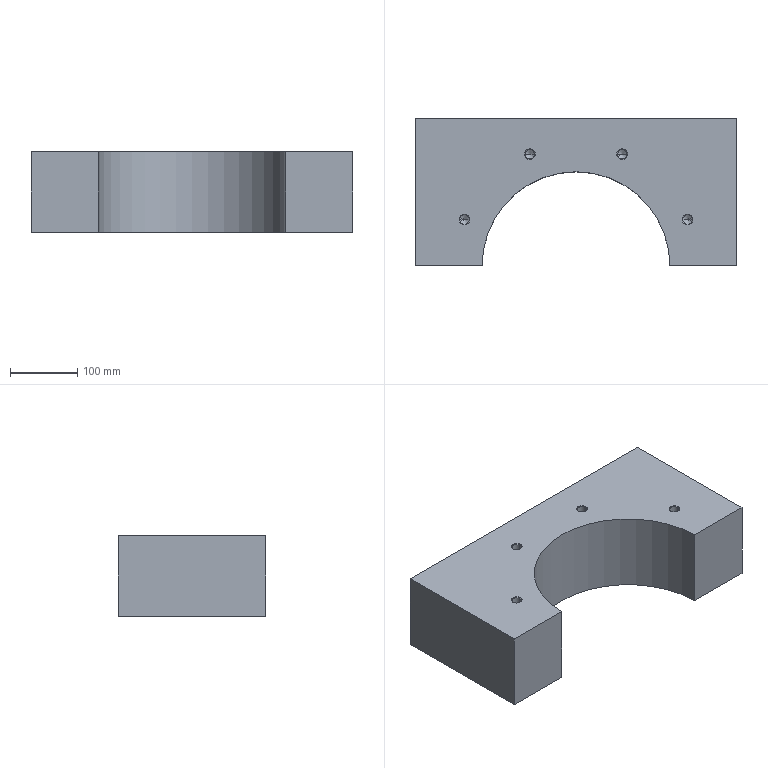Part | SolidWorks | features Extrusion 1, HoleWzd 1, RefAxis 1 | 1 solid | 32 faces | box 480 x 220 x 120 mm | volume 8956950 mm3 | cone 16 | cylinder 9 | plane 7 | commonest cylinder face diameters 14 x8 280 x1
STEP:
#1=CARTESIAN_POINT('',(-173.298,68.883,118.975));
#2=VERTEX_POINT('',#1);
#3=CARTESIAN_POINT('',(-159.298,68.883,118.975));
#4=VERTEX_POINT('',#3);
#5=CARTESIAN_POINT('',(-166.298,68.883,118.975));
#6=DIRECTION('',(0.,0.,1.));
#7=DIRECTION('',(1.,0.,0.));
#8=AXIS2_PLACEMENT_3D('',#5,#6,#7);
#9=CIRCLE('',#8,7.);
#10=EDGE_CURVE('',#2,#4,#9,.T.);
#11=ORIENTED_EDGE('',*,*,#10,.F.);
#12=CARTESIAN_POINT('',(-174.323,68.883,120.));
#13=VERTEX_POINT('',#12);
#14=CARTESIAN_POINT('',(-174.323,68.883,120.));
#15=DIRECTION('',(-0.7071,0.,0.7071));
#16=VECTOR('',#15,1000.);
#17=LINE('',#14,#16);
#18=EDGE_CURVE('',#2,#13,#17,.T.);
#19=ORIENTED_EDGE('',*,*,#18,.T.);
#20=CARTESIAN_POINT('',(-158.273,68.883,120.));
#21=VERTEX_POINT('',#20);
#22=CARTESIAN_POINT('',(-166.298,68.883,120.));
#23=DIRECTION('',(0.,0.,1.));
#24=DIRECTION('',(1.,0.,0.));
#25=AXIS2_PLACEMENT_3D('',#22,#23,#24);
#26=CIRCLE('',#25,8.025);
#27=EDGE_CURVE('',#13,#21,#26,.T.);
#28=ORIENTED_EDGE('',*,*,#27,.T.);
#29=CARTESIAN_POINT('',(-158.273,68.883,120.));
#30=DIRECTION('',(0.7071,0.,0.7071));
#31=VECTOR('',#30,1000.);
#32=LINE('',#29,#31);
#33=EDGE_CURVE('',#4,#21,#32,.T.);
#34=ORIENTED_EDGE('',*,*,#33,.F.);
#35=EDGE_LOOP('',(#11,#19,#28,#34));
#36=FACE_OUTER_BOUND('',#35,.T.);
#37=CARTESIAN_POINT('',(-166.298,68.883,120.));
#38=DIRECTION('',(0.,0.,1.));
#39=DIRECTION('',(1.,0.,0.));
#40=AXIS2_PLACEMENT_3D('',#37,#38,#39);
#41=CONICAL_SURFACE('',#40,8.025,0.7854);
#42=ADVANCED_FACE('',(#36),#41,.F.);
#43=CARTESIAN_POINT('',(-173.298,68.883,88.206));
#44=VERTEX_POINT('',#43);
#45=CARTESIAN_POINT('',(-159.298,68.883,88.206));
#46=VERTEX_POINT('',#45);
#47=CARTESIAN_POINT('',(-166.298,68.883,88.206));
#48=DIRECTION('',(0.,0.,1.));
#49=DIRECTION('',(1.,0.,0.));
#50=AXIS2_PLACEMENT_3D('',#47,#48,#49);
#51=CIRCLE('',#50,7.);
#52=EDGE_CURVE('',#44,#46,#51,.T.);
#53=ORIENTED_EDGE('',*,*,#52,.F.);
#54=CARTESIAN_POINT('',(-173.298,68.883,120.));
#55=DIRECTION('',(0.,0.,1.));
#56=VECTOR('',#55,1000.);
#57=LINE('',#54,#56);
#58=EDGE_CURVE('',#44,#2,#57,.T.);
#59=ORIENTED_EDGE('',*,*,#58,.T.);
#60=ORIENTED_EDGE('',*,*,#10,.T.);
#61=CARTESIAN_POINT('',(-159.298,68.883,120.));
#62=DIRECTION('',(0.,0.,1.));
#63=VECTOR('',#62,1000.);
#64=LINE('',#61,#63);
#65=EDGE_CURVE('',#46,#4,#64,.T.);
#66=ORIENTED_EDGE('',*,*,#65,.F.);
#67=EDGE_LOOP('',(#53,#59,#60,#66));
#68=FACE_OUTER_BOUND('',#67,.T.);
#69=CARTESIAN_POINT('',(-166.298,68.883,120.));
#70=DIRECTION('',(0.,0.,1.));
#71=DIRECTION('',(1.,0.,0.));
#72=AXIS2_PLACEMENT_3D('',#69,#70,#71);
#73=CYLINDRICAL_SURFACE('',#72,7.);
#74=ADVANCED_FACE('',(#68),#73,.F.);
#75=CARTESIAN_POINT('',(-166.298,68.883,84.));
#76=VERTEX_POINT('',#75);
#77=CARTESIAN_POINT('',(-159.298,68.883,88.206));
#78=DIRECTION('',(0.8572,0.,0.515));
#79=VECTOR('',#78,1000.);
#80=LINE('',#77,#79);
#81=EDGE_CURVE('',#76,#46,#80,.T.);
#82=ORIENTED_EDGE('',*,*,#81,.F.);
#83=CARTESIAN_POINT('',(-173.298,68.883,88.206));
#84=DIRECTION('',(-0.8572,0.,0.515));
#85=VECTOR('',#84,1000.);
#86=LINE('',#83,#85);
#87=EDGE_CURVE('',#76,#44,#86,.T.);
#88=ORIENTED_EDGE('',*,*,#87,.T.);
#89=ORIENTED_EDGE('',*,*,#52,.T.);
#90=EDGE_LOOP('',(#82,#88,#89));
#91=FACE_OUTER_BOUND('',#90,.T.);
#92=CARTESIAN_POINT('',(-166.298,68.883,88.206));
#93=DIRECTION('',(0.,0.,1.));
#94=DIRECTION('',(1.,0.,0.));
#95=AXIS2_PLACEMENT_3D('',#92,#93,#94);
#96=CONICAL_SURFACE('',#95,7.,1.03);
#97=ADVANCED_FACE('',(#91),#96,.F.);
#98=CARTESIAN_POINT('',(-75.883,166.298,118.975));
#99=VERTEX_POINT('',#98);
#100=CARTESIAN_POINT('',(-61.883,166.298,118.975));
#101=VERTEX_POINT('',#100);
#102=CARTESIAN_POINT('',(-68.883,166.298,118.975));
#103=DIRECTION('',(0.,0.,1.));
#104=DIRECTION('',(1.,0.,0.));
#105=AXIS2_PLACEMENT_3D('',#102,#103,#104);
#106=CIRCLE('',#105,7.);
#107=EDGE_CURVE('',#99,#101,#106,.T.);
#108=ORIENTED_EDGE('',*,*,#107,.F.);
#109=CARTESIAN_POINT('',(-76.908,166.298,120.));
#110=VERTEX_POINT('',#109);
#111=CARTESIAN_POINT('',(-76.908,166.298,120.));
#112=DIRECTION('',(-0.7071,0.,0.7071));
#113=VECTOR('',#112,1000.);
#114=LINE('',#111,#113);
#115=EDGE_CURVE('',#99,#110,#114,.T.);
#116=ORIENTED_EDGE('',*,*,#115,.T.);
#117=CARTESIAN_POINT('',(-60.858,166.298,120.));
#118=VERTEX_POINT('',#117);
#119=CARTESIAN_POINT('',(-68.883,166.298,120.));
#120=DIRECTION('',(0.,0.,1.));
#121=DIRECTION('',(1.,0.,0.));
#122=AXIS2_PLACEMENT_3D('',#119,#120,#121);
#123=CIRCLE('',#122,8.025);
#124=EDGE_CURVE('',#110,#118,#123,.T.);
#125=ORIENTED_EDGE('',*,*,#124,.T.);
#126=CARTESIAN_POINT('',(-60.858,166.298,120.));
#127=DIRECTION('',(0.7071,0.,0.7071));
#128=VECTOR('',#127,1000.);
#129=LINE('',#126,#128);
#130=EDGE_CURVE('',#101,#118,#129,.T.);
#131=ORIENTED_EDGE('',*,*,#130,.F.);
#132=EDGE_LOOP('',(#108,#116,#125,#131));
#133=FACE_OUTER_BOUND('',#132,.T.);
#134=CARTESIAN_POINT('',(-68.883,166.298,120.));
#135=DIRECTION('',(0.,0.,1.));
#136=DIRECTION('',(1.,0.,0.));
#137=AXIS2_PLACEMENT_3D('',#134,#135,#136);
#138=CONICAL_SURFACE('',#137,8.025,0.7854);
#139=ADVANCED_FACE('',(#133),#138,.F.);
#140=CARTESIAN_POINT('',(-75.883,166.298,88.206));
#141=VERTEX_POINT('',#140);
#142=CARTESIAN_POINT('',(-61.883,166.298,88.206));
#143=VERTEX_POINT('',#142);
#144=CARTESIAN_POINT('',(-68.883,166.298,88.206));
#145=DIRECTION('',(0.,0.,1.));
#146=DIRECTION('',(1.,0.,0.));
#147=AXIS2_PLACEMENT_3D('',#144,#145,#146);
#148=CIRCLE('',#147,7.);
#149=EDGE_CURVE('',#141,#143,#148,.T.);
#150=ORIENTED_EDGE('',*,*,#149,.F.);
#151=CARTESIAN_POINT('',(-75.883,166.298,120.));
#152=DIRECTION('',(0.,0.,1.));
#153=VECTOR('',#152,1000.);
#154=LINE('',#151,#153);
#155=EDGE_CURVE('',#141,#99,#154,.T.);
#156=ORIENTED_EDGE('',*,*,#155,.T.);
#157=ORIENTED_EDGE('',*,*,#107,.T.);
#158=CARTESIAN_POINT('',(-61.883,166.298,120.));
#159=DIRECTION('',(0.,0.,1.));
#160=VECTOR('',#159,1000.);
#161=LINE('',#158,#160);
#162=EDGE_CURVE('',#143,#101,#161,.T.);
#163=ORIENTED_EDGE('',*,*,#162,.F.);
#164=EDGE_LOOP('',(#150,#156,#157,#163));
#165=FACE_OUTER_BOUND('',#164,.T.);
#166=CARTESIAN_POINT('',(-68.883,166.298,120.));
#167=DIRECTION('',(0.,0.,1.));
#168=DIRECTION('',(1.,0.,0.));
#169=AXIS2_PLACEMENT_3D('',#166,#167,#168);
#170=CYLINDRICAL_SURFACE('',#169,7.);
#171=ADVANCED_FACE('',(#165),#170,.F.);
#172=CARTESIAN_POINT('',(-68.883,166.298,84.));
#173=VERTEX_POINT('',#172);
#174=CARTESIAN_POINT('',(-61.883,166.298,88.206));
#175=DIRECTION('',(0.8572,0.,0.515));
#176=VECTOR('',#175,1000.);
#177=LINE('',#174,#176);
#178=EDGE_CURVE('',#173,#143,#177,.T.);
#179=ORIENTED_EDGE('',*,*,#178,.F.);
#180=CARTESIAN_POINT('',(-75.883,166.298,88.206));
#181=DIRECTION('',(-0.8572,0.,0.515));
#182=VECTOR('',#181,1000.);
#183=LINE('',#180,#182);
#184=EDGE_CURVE('',#173,#141,#183,.T.);
#185=ORIENTED_EDGE('',*,*,#184,.T.);
#186=ORIENTED_EDGE('',*,*,#149,.T.);
#187=EDGE_LOOP('',(#179,#185,#186));
#188=FACE_OUTER_BOUND('',#187,.T.);
#189=CARTESIAN_POINT('',(-68.883,166.298,88.206));
#190=DIRECTION('',(0.,0.,1.));
#191=DIRECTION('',(1.,0.,0.));
#192=AXIS2_PLACEMENT_3D('',#189,#190,#191);
#193=CONICAL_SURFACE('',#192,7.,1.03);
#194=ADVANCED_FACE('',(#188),#193,.F.);
#195=CARTESIAN_POINT('',(61.883,166.298,118.975));
#196=VERTEX_POINT('',#195);
#197=CARTESIAN_POINT('',(75.883,166.298,118.975));
#198=VERTEX_POINT('',#197);
#199=CARTESIAN_POINT('',(68.883,166.298,118.975));
#200=DIRECTION('',(0.,0.,1.));
#201=DIRECTION('',(1.,0.,0.));
#202=AXIS2_PLACEMENT_3D('',#199,#200,#201);
#203=CIRCLE('',#202,7.);
#204=EDGE_CURVE('',#196,#198,#203,.T.);
#205=ORIENTED_EDGE('',*,*,#204,.F.);
#206=CARTESIAN_POINT('',(60.858,166.298,120.));
#207=VERTEX_POINT('',#206);
#208=CARTESIAN_POINT('',(60.858,166.298,120.));
#209=DIRECTION('',(-0.7071,0.,0.7071));
#210=VECTOR('',#209,1000.);
#211=LINE('',#208,#210);
#212=EDGE_CURVE('',#196,#207,#211,.T.);
#213=ORIENTED_EDGE('',*,*,#212,.T.);
#214=CARTESIAN_POINT('',(76.908,166.298,120.));
#215=VERTEX_POINT('',#214);
#216=CARTESIAN_POINT('',(68.883,166.298,120.));
#217=DIRECTION('',(0.,0.,1.));
#218=DIRECTION('',(1.,0.,0.));
#219=AXIS2_PLACEMENT_3D('',#216,#217,#218);
#220=CIRCLE('',#219,8.025);
#221=EDGE_CURVE('',#207,#215,#220,.T.);
#222=ORIENTED_EDGE('',*,*,#221,.T.);
#223=CARTESIAN_POINT('',(76.908,166.298,120.));
#224=DIRECTION('',(0.7071,0.,0.7071));
#225=VECTOR('',#224,1000.);
#226=LINE('',#223,#225);
#227=EDGE_CURVE('',#198,#215,#226,.T.);
#228=ORIENTED_EDGE('',*,*,#227,.F.);
#229=EDGE_LOOP('',(#205,#213,#222,#228));
#230=FACE_OUTER_BOUND('',#229,.T.);
#231=CARTESIAN_POINT('',(68.883,166.298,120.));
#232=DIRECTION('',(0.,0.,1.));
#233=DIRECTION('',(1.,0.,0.));
#234=AXIS2_PLACEMENT_3D('',#231,#232,#233);
#235=CONICAL_SURFACE('',#234,8.025,0.7854);
#236=ADVANCED_FACE('',(#230),#235,.F.);
#237=CARTESIAN_POINT('',(61.883,166.298,88.206));
#238=VERTEX_POINT('',#237);
#239=CARTESIAN_POINT('',(75.883,166.298,88.206));
#240=VERTEX_POINT('',#239);
#241=CARTESIAN_POINT('',(68.883,166.298,88.206));
#242=DIRECTION('',(0.,0.,1.));
#243=DIRECTION('',(1.,0.,0.));
#244=AXIS2_PLACEMENT_3D('',#241,#242,#243);
#245=CIRCLE('',#244,7.);
#246=EDGE_CURVE('',#238,#240,#245,.T.);
#247=ORIENTED_EDGE('',*,*,#246,.F.);
#248=CARTESIAN_POINT('',(61.883,166.298,120.));
#249=DIRECTION('',(0.,0.,1.));
#250=VECTOR('',#249,1000.);
#251=LINE('',#248,#250);
#252=EDGE_CURVE('',#238,#196,#251,.T.);
#253=ORIENTED_EDGE('',*,*,#252,.T.);
#254=ORIENTED_EDGE('',*,*,#204,.T.);
#255=CARTESIAN_POINT('',(75.883,166.298,120.));
#256=DIRECTION('',(0.,0.,1.));
#257=VECTOR('',#256,1000.);
#258=LINE('',#255,#257);
#259=EDGE_CURVE('',#240,#198,#258,.T.);
#260=ORIENTED_EDGE('',*,*,#259,.F.);
#261=EDGE_LOOP('',(#247,#253,#254,#260));
#262=FACE_OUTER_BOUND('',#261,.T.);
#263=CARTESIAN_POINT('',(68.883,166.298,120.));
#264=DIRECTION('',(0.,0.,1.));
#265=DIRECTION('',(1.,0.,0.));
#266=AXIS2_PLACEMENT_3D('',#263,#264,#265);
#267=CYLINDRICAL_SURFACE('',#266,7.);
#268=ADVANCED_FACE('',(#262),#267,.F.);
#269=CARTESIAN_POINT('',(68.883,166.298,84.));
#270=VERTEX_POINT('',#269);
#271=CARTESIAN_POINT('',(75.883,166.298,88.206));
#272=DIRECTION('',(0.8572,0.,0.515));
#273=VECTOR('',#272,1000.);
#274=LINE('',#271,#273);
#275=EDGE_CURVE('',#270,#240,#274,.T.);
#276=ORIENTED_EDGE('',*,*,#275,.F.);
#277=CARTESIAN_POINT('',(61.883,166.298,88.206));
#278=DIRECTION('',(-0.8572,0.,0.515));
#279=VECTOR('',#278,1000.);
#280=LINE('',#277,#279);
#281=EDGE_CURVE('',#270,#238,#280,.T.);
#282=ORIENTED_EDGE('',*,*,#281,.T.);
#283=ORIENTED_EDGE('',*,*,#246,.T.);
#284=EDGE_LOOP('',(#276,#282,#283));
#285=FACE_OUTER_BOUND('',#284,.T.);
#286=CARTESIAN_POINT('',(68.883,166.298,88.206));
#287=DIRECTION('',(0.,0.,1.));
#288=DIRECTION('',(1.,0.,0.));
#289=AXIS2_PLACEMENT_3D('',#286,#287,#288);
#290=CONICAL_SURFACE('',#289,7.,1.03);
#291=ADVANCED_FACE('',(#285),#290,.F.);
#292=CARTESIAN_POINT('',(159.298,68.883,118.975));
#293=VERTEX_POINT('',#292);
#294=CARTESIAN_POINT('',(173.298,68.883,118.975));
#295=VERTEX_POINT('',#294);
#296=CARTESIAN_POINT('',(166.298,68.883,118.975));
#297=DIRECTION('',(0.,0.,1.));
#298=DIRECTION('',(1.,0.,0.));
#299=AXIS2_PLACEMENT_3D('',#296,#297,#298);
#300=CIRCLE('',#299,7.);
#301=EDGE_CURVE('',#293,#295,#300,.T.);
#302=ORIENTED_EDGE('',*,*,#301,.F.);
#303=CARTESIAN_POINT('',(158.273,68.883,120.));
#304=VERTEX_POINT('',#303);
#305=CARTESIAN_POINT('',(158.273,68.883,120.));
#306=DIRECTION('',(-0.7071,0.,0.7071));
#307=VECTOR('',#306,1000.);
#308=LINE('',#305,#307);
#309=EDGE_CURVE('',#293,#304,#308,.T.);
#310=ORIENTED_EDGE('',*,*,#309,.T.);
#311=CARTESIAN_POINT('',(174.323,68.883,120.));
#312=VERTEX_POINT('',#311);
#313=CARTESIAN_POINT('',(166.298,68.883,120.));
#314=DIRECTION('',(0.,0.,1.));
#315=DIRECTION('',(1.,0.,0.));
#316=AXIS2_PLACEMENT_3D('',#313,#314,#315);
#317=CIRCLE('',#316,8.025);
#318=EDGE_CURVE('',#304,#312,#317,.T.);
#319=ORIENTED_EDGE('',*,*,#318,.T.);
#320=CARTESIAN_POINT('',(174.323,68.883,120.));
#321=DIRECTION('',(0.7071,0.,0.7071));
#322=VECTOR('',#321,1000.);
#323=LINE('',#320,#322);
#324=EDGE_CURVE('',#295,#312,#323,.T.);
#325=ORIENTED_EDGE('',*,*,#324,.F.);
#326=EDGE_LOOP('',(#302,#310,#319,#325));
#327=FACE_OUTER_BOUND('',#326,.T.);
#328=CARTESIAN_POINT('',(166.298,68.883,120.));
#329=DIRECTION('',(0.,0.,1.));
#330=DIRECTION('',(1.,0.,0.));
#331=AXIS2_PLACEMENT_3D('',#328,#329,#330);
#332=CONICAL_SURFACE('',#331,8.025,0.7854);
#333=ADVANCED_FACE('',(#327),#332,.F.);
#334=CARTESIAN_POINT('',(159.298,68.883,88.206));
#335=VERTEX_POINT('',#334);
#336=CARTESIAN_POINT('',(173.298,68.883,88.206));
#337=VERTEX_POINT('',#336);
#338=CARTESIAN_POINT('',(166.298,68.883,88.206));
#339=DIRECTION('',(0.,0.,1.));
#340=DIRECTION('',(1.,0.,0.));
#341=AXIS2_PLACEMENT_3D('',#338,#339,#340);
#342=CIRCLE('',#341,7.);
#343=EDGE_CURVE('',#335,#337,#342,.T.);
#344=ORIENTED_EDGE('',*,*,#343,.F.);
#345=CARTESIAN_POINT('',(159.298,68.883,120.));
#346=DIRECTION('',(0.,0.,1.));
#347=VECTOR('',#346,1000.);
#348=LINE('',#345,#347);
#349=EDGE_CURVE('',#335,#293,#348,.T.);
#350=ORIENTED_EDGE('',*,*,#349,.T.);
#351=ORIENTED_EDGE('',*,*,#301,.T.);
#352=CARTESIAN_POINT('',(173.298,68.883,120.));
#353=DIRECTION('',(0.,0.,1.));
#354=VECTOR('',#353,1000.);
#355=LINE('',#352,#354);
#356=EDGE_CURVE('',#337,#295,#355,.T.);
#357=ORIENTED_EDGE('',*,*,#356,.F.);
#358=EDGE_LOOP('',(#344,#350,#351,#357));
#359=FACE_OUTER_BOUND('',#358,.T.);
#360=CARTESIAN_POINT('',(166.298,68.883,120.));
#361=DIRECTION('',(0.,0.,1.));
#362=DIRECTION('',(1.,0.,0.));
#363=AXIS2_PLACEMENT_3D('',#360,#361,#362);
#364=CYLINDRICAL_SURFACE('',#363,7.);
#365=ADVANCED_FACE('',(#359),#364,.F.);
#366=CARTESIAN_POINT('',(166.298,68.883,84.));
#367=VERTEX_POINT('',#366);
#368=CARTESIAN_POINT('',(173.298,68.883,88.206));
#369=DIRECTION('',(0.8572,0.,0.515));
#370=VECTOR('',#369,1000.);
#371=LINE('',#368,#370);
#372=EDGE_CURVE('',#367,#337,#371,.T.);
#373=ORIENTED_EDGE('',*,*,#372,.F.);
#374=CARTESIAN_POINT('',(159.298,68.883,88.206));
#375=DIRECTION('',(-0.8572,0.,0.515));
#376=VECTOR('',#375,1000.);
#377=LINE('',#374,#376);
#378=EDGE_CURVE('',#367,#335,#377,.T.);
#379=ORIENTED_EDGE('',*,*,#378,.T.);
#380=ORIENTED_EDGE('',*,*,#343,.T.);
#381=EDGE_LOOP('',(#373,#379,#380));
#382=FACE_OUTER_BOUND('',#381,.T.);
#383=CARTESIAN_POINT('',(166.298,68.883,88.206));
#384=DIRECTION('',(0.,0.,1.));
#385=DIRECTION('',(1.,0.,0.));
#386=AXIS2_PLACEMENT_3D('',#383,#384,#385);
#387=CONICAL_SURFACE('',#386,7.,1.03);
#388=ADVANCED_FACE('',(#382),#387,.F.);
#389=CARTESIAN_POINT('',(140.,0.,0.));
#390=VERTEX_POINT('',#389);
#391=CARTESIAN_POINT('',(240.,0.,0.));
#392=VERTEX_POINT('',#391);
#393=CARTESIAN_POINT('',(140.,0.,0.));
#394=DIRECTION('',(1.,0.,0.));
#395=VECTOR('',#394,1000.);
#396=LINE('',#393,#395);
#397=EDGE_CURVE('',#390,#392,#396,.T.);
#398=ORIENTED_EDGE('',*,*,#397,.T.);
#399=CARTESIAN_POINT('',(240.,0.,120.));
#400=VERTEX_POINT('',#399);
#401=CARTESIAN_POINT('',(240.,0.,120.));
#402=DIRECTION('',(0.,0.,-1.));
#403=VECTOR('',#402,1000.);
#404=LINE('',#401,#403);
#405=EDGE_CURVE('',#400,#392,#404,.T.);
#406=ORIENTED_EDGE('',*,*,#405,.F.);
#407=CARTESIAN_POINT('',(140.,0.,120.));
#408=VERTEX_POINT('',#407);
#409=CARTESIAN_POINT('',(140.,0.,120.));
#410=DIRECTION('',(1.,0.,0.));
#411=VECTOR('',#410,1000.);
#412=LINE('',#409,#411);
#413=EDGE_CURVE('',#408,#400,#412,.T.);
#414=ORIENTED_EDGE('',*,*,#413,.F.);
#415=CARTESIAN_POINT('',(140.,0.,120.));
#416=DIRECTION('',(0.,0.,-1.));
#417=VECTOR('',#416,1000.);
#418=LINE('',#415,#417);
#419=EDGE_CURVE('',#408,#390,#418,.T.);
#420=ORIENTED_EDGE('',*,*,#419,.T.);
#421=EDGE_LOOP('',(#398,#406,#414,#420));
#422=FACE_OUTER_BOUND('',#421,.T.);
#423=CARTESIAN_POINT('',(140.,0.,120.));
#424=DIRECTION('',(0.,1.,0.));
#425=DIRECTION('',(0.,0.,1.));
#426=AXIS2_PLACEMENT_3D('',#423,#424,#425);
#427=PLANE('',#426);
#428=ADVANCED_FACE('',(#422),#427,.F.);
#429=CARTESIAN_POINT('',(240.,220.,0.));
#430=VERTEX_POINT('',#429);
#431=CARTESIAN_POINT('',(240.,220.,0.));
#432=DIRECTION('',(0.,1.,0.));
#433=VECTOR('',#432,1000.);
#434=LINE('',#431,#433);
#435=EDGE_CURVE('',#392,#430,#434,.T.);
#436=ORIENTED_EDGE('',*,*,#435,.T.);
#437=CARTESIAN_POINT('',(240.,220.,120.));
#438=VERTEX_POINT('',#437);
#439=CARTESIAN_POINT('',(240.,220.,120.));
#440=DIRECTION('',(0.,0.,-1.));
#441=VECTOR('',#440,1000.);
#442=LINE('',#439,#441);
#443=EDGE_CURVE('',#438,#430,#442,.T.);
#444=ORIENTED_EDGE('',*,*,#443,.F.);
#445=CARTESIAN_POINT('',(240.,220.,120.));
#446=DIRECTION('',(0.,1.,0.));
#447=VECTOR('',#446,1000.);
#448=LINE('',#445,#447);
#449=EDGE_CURVE('',#400,#438,#448,.T.);
#450=ORIENTED_EDGE('',*,*,#449,.F.);
#451=ORIENTED_EDGE('',*,*,#405,.T.);
#452=EDGE_LOOP('',(#436,#444,#450,#451));
#453=FACE_OUTER_BOUND('',#452,.T.);
#454=CARTESIAN_POINT('',(240.,220.,120.));
#455=DIRECTION('',(-1.,0.,0.));
#456=DIRECTION('',(0.,-1.,0.));
#457=AXIS2_PLACEMENT_3D('',#454,#455,#456);
#458=PLANE('',#457);
#459=ADVANCED_FACE('',(#453),#458,.F.);
#460=CARTESIAN_POINT('',(-240.,220.,0.));
#461=VERTEX_POINT('',#460);
#462=CARTESIAN_POINT('',(-240.,220.,0.));
#463=DIRECTION('',(-1.,0.,0.));
#464=VECTOR('',#463,1000.);
#465=LINE('',#462,#464);
#466=EDGE_CURVE('',#430,#461,#465,.T.);
#467=ORIENTED_EDGE('',*,*,#466,.T.);
#468=CARTESIAN_POINT('',(-240.,220.,120.));
#469=VERTEX_POINT('',#468);
#470=CARTESIAN_POINT('',(-240.,220.,120.));
#471=DIRECTION('',(0.,0.,-1.));
#472=VECTOR('',#471,1000.);
#473=LINE('',#470,#472);
#474=EDGE_CURVE('',#469,#461,#473,.T.);
#475=ORIENTED_EDGE('',*,*,#474,.F.);
#476=CARTESIAN_POINT('',(-240.,220.,120.));
#477=DIRECTION('',(-1.,0.,0.));
#478=VECTOR('',#477,1000.);
#479=LINE('',#476,#478);
#480=EDGE_CURVE('',#438,#469,#479,.T.);
#481=ORIENTED_EDGE('',*,*,#480,.F.);
#482=ORIENTED_EDGE('',*,*,#443,.T.);
#483=EDGE_LOOP('',(#467,#475,#481,#482));
#484=FACE_OUTER_BOUND('',#483,.T.);
#485=CARTESIAN_POINT('',(-240.,220.,120.));
#486=DIRECTION('',(0.,-1.,0.));
#487=DIRECTION('',(0.,0.,-1.));
#488=AXIS2_PLACEMENT_3D('',#485,#486,#487);
#489=PLANE('',#488);
#490=ADVANCED_FACE('',(#484),#489,.F.);
#491=CARTESIAN_POINT('',(-240.,0.,0.));
#492=VERTEX_POINT('',#491);
#493=CARTESIAN_POINT('',(-240.,220.,0.));
#494=DIRECTION('',(0.,-1.,0.));
#495=VECTOR('',#494,1000.);
#496=LINE('',#493,#495);
#497=EDGE_CURVE('',#461,#492,#496,.T.);
#498=ORIENTED_EDGE('',*,*,#497,.T.);
#499=CARTESIAN_POINT('',(-240.,0.,120.));
#500=VERTEX_POINT('',#499);
#501=CARTESIAN_POINT('',(-240.,0.,120.));
#502=DIRECTION('',(0.,0.,-1.));
#503=VECTOR('',#502,1000.);
#504=LINE('',#501,#503);
#505=EDGE_CURVE('',#500,#492,#504,.T.);
#506=ORIENTED_EDGE('',*,*,#505,.F.);
#507=CARTESIAN_POINT('',(-240.,220.,120.));
#508=DIRECTION('',(0.,-1.,0.));
#509=VECTOR('',#508,1000.);
#510=LINE('',#507,#509);
#511=EDGE_CURVE('',#469,#500,#510,.T.);
#512=ORIENTED_EDGE('',*,*,#511,.F.);
#513=ORIENTED_EDGE('',*,*,#474,.T.);
#514=EDGE_LOOP('',(#498,#506,#512,#513));
#515=FACE_OUTER_BOUND('',#514,.T.);
#516=CARTESIAN_POINT('',(-240.,220.,120.));
#517=DIRECTION('',(1.,0.,0.));
#518=DIRECTION('',(0.,1.,0.));
#519=AXIS2_PLACEMENT_3D('',#516,#517,#518);
#520=PLANE('',#519);
#521=ADVANCED_FACE('',(#515),#520,.F.);
#522=CARTESIAN_POINT('',(-140.,0.,0.));
#523=VERTEX_POINT('',#522);
#524=CARTESIAN_POINT('',(-240.,0.,0.));
#525=DIRECTION('',(1.,0.,0.));
#526=VECTOR('',#525,1000.);
#527=LINE('',#524,#526);
#528=EDGE_CURVE('',#492,#523,#527,.T.);
#529=ORIENTED_EDGE('',*,*,#528,.T.);
#530=CARTESIAN_POINT('',(-140.,0.,120.));
#531=VERTEX_POINT('',#530);
#532=CARTESIAN_POINT('',(-140.,0.,120.));
#533=DIRECTION('',(0.,0.,-1.));
#534=VECTOR('',#533,1000.);
#535=LINE('',#532,#534);
#536=EDGE_CURVE('',#531,#523,#535,.T.);
#537=ORIENTED_EDGE('',*,*,#536,.F.);
#538=CARTESIAN_POINT('',(-240.,0.,120.));
#539=DIRECTION('',(1.,0.,0.));
#540=VECTOR('',#539,1000.);
#541=LINE('',#538,#540);
#542=EDGE_CURVE('',#500,#531,#541,.T.);
#543=ORIENTED_EDGE('',*,*,#542,.F.);
#544=ORIENTED_EDGE('',*,*,#505,.T.);
#545=EDGE_LOOP('',(#529,#537,#543,#544));
#546=FACE_OUTER_BOUND('',#545,.T.);
#547=CARTESIAN_POINT('',(-240.,0.,120.));
#548=DIRECTION('',(0.,1.,0.));
#549=DIRECTION('',(0.,0.,1.));
#550=AXIS2_PLACEMENT_3D('',#547,#548,#549);
#551=PLANE('',#550);
#552=ADVANCED_FACE('',(#546),#551,.F.);
#553=CARTESIAN_POINT('',(0.,0.,0.));
#554=DIRECTION('',(0.,0.,-1.));
#555=DIRECTION('',(1.,0.,0.));
#556=AXIS2_PLACEMENT_3D('',#553,#554,#555);
#557=CIRCLE('',#556,140.);
#558=EDGE_CURVE('',#523,#390,#557,.T.);
#559=ORIENTED_EDGE('',*,*,#558,.T.);
#560=ORIENTED_EDGE('',*,*,#419,.F.);
#561=CARTESIAN_POINT('',(0.,0.,120.));
#562=DIRECTION('',(0.,0.,-1.));
#563=DIRECTION('',(1.,0.,0.));
#564=AXIS2_PLACEMENT_3D('',#561,#562,#563);
#565=CIRCLE('',#564,140.);
#566=EDGE_CURVE('',#531,#408,#565,.T.);
#567=ORIENTED_EDGE('',*,*,#566,.F.);
#568=ORIENTED_EDGE('',*,*,#536,.T.);
#569=EDGE_LOOP('',(#559,#560,#567,#568));
#570=FACE_OUTER_BOUND('',#569,.T.);
#571=CARTESIAN_POINT('',(0.,0.,120.));
#572=DIRECTION('',(0.,0.,-1.));
#573=DIRECTION('',(-1.,0.,0.));
#574=AXIS2_PLACEMENT_3D('',#571,#572,#573);
#575=CYLINDRICAL_SURFACE('',#574,140.);
#576=ADVANCED_FACE('',(#570),#575,.F.);
#577=CARTESIAN_POINT('',(-166.298,68.883,120.));
#578=DIRECTION('',(0.,0.,1.));
#579=DIRECTION('',(1.,0.,0.));
#580=AXIS2_PLACEMENT_3D('',#577,#578,#579);
#581=CIRCLE('',#580,8.025);
#582=EDGE_CURVE('',#21,#13,#581,.T.);
#583=ORIENTED_EDGE('',*,*,#582,.F.);
#584=ORIENTED_EDGE('',*,*,#27,.F.);
#585=EDGE_LOOP('',(#583,#584));
#586=FACE_BOUND('',#585,.T.);
#587=CARTESIAN_POINT('',(-68.883,166.298,120.));
#588=DIRECTION('',(0.,0.,1.));
#589=DIRECTION('',(1.,0.,0.));
#590=AXIS2_PLACEMENT_3D('',#587,#588,#589);
#591=CIRCLE('',#590,8.025);
#592=EDGE_CURVE('',#118,#110,#591,.T.);
#593=ORIENTED_EDGE('',*,*,#592,.F.);
#594=ORIENTED_EDGE('',*,*,#124,.F.);
#595=EDGE_LOOP('',(#593,#594));
#596=FACE_BOUND('',#595,.T.);
#597=CARTESIAN_POINT('',(68.883,166.298,120.));
#598=DIRECTION('',(0.,0.,1.));
#599=DIRECTION('',(1.,0.,0.));
#600=AXIS2_PLACEMENT_3D('',#597,#598,#599);
#601=CIRCLE('',#600,8.025);
#602=EDGE_CURVE('',#215,#207,#601,.T.);
#603=ORIENTED_EDGE('',*,*,#602,.F.);
#604=ORIENTED_EDGE('',*,*,#221,.F.);
#605=EDGE_LOOP('',(#603,#604));
#606=FACE_BOUND('',#605,.T.);
#607=CARTESIAN_POINT('',(166.298,68.883,120.));
#608=DIRECTION('',(0.,0.,1.));
#609=DIRECTION('',(1.,0.,0.));
#610=AXIS2_PLACEMENT_3D('',#607,#608,#609);
#611=CIRCLE('',#610,8.025);
#612=EDGE_CURVE('',#312,#304,#611,.T.);
#613=ORIENTED_EDGE('',*,*,#612,.F.);
#614=ORIENTED_EDGE('',*,*,#318,.F.);
#615=EDGE_LOOP('',(#613,#614));
#616=FACE_BOUND('',#615,.T.);
#617=ORIENTED_EDGE('',*,*,#413,.T.);
#618=ORIENTED_EDGE('',*,*,#449,.T.);
#619=ORIENTED_EDGE('',*,*,#480,.T.);
#620=ORIENTED_EDGE('',*,*,#511,.T.);
#621=ORIENTED_EDGE('',*,*,#542,.T.);
#622=ORIENTED_EDGE('',*,*,#566,.T.);
#623=EDGE_LOOP('',(#617,#618,#619,#620,#621,#622));
#624=FACE_OUTER_BOUND('',#623,.T.);
#625=CARTESIAN_POINT('',(0.,0.,120.));
#626=DIRECTION('',(0.,0.,1.));
#627=DIRECTION('',(1.,0.,0.));
#628=AXIS2_PLACEMENT_3D('',#625,#626,#627);
#629=PLANE('',#628);
#630=ADVANCED_FACE('',(#586,#596,#606,#616,#624),#629,.T.);
#631=ORIENTED_EDGE('',*,*,#397,.F.);
#632=ORIENTED_EDGE('',*,*,#558,.F.);
#633=ORIENTED_EDGE('',*,*,#528,.F.);
#634=ORIENTED_EDGE('',*,*,#497,.F.);
#635=ORIENTED_EDGE('',*,*,#466,.F.);
#636=ORIENTED_EDGE('',*,*,#435,.F.);
#637=EDGE_LOOP('',(#631,#632,#633,#634,#635,#636));
#638=FACE_OUTER_BOUND('',#637,.T.);
#639=CARTESIAN_POINT('',(0.,0.,0.));
#640=DIRECTION('',(0.,0.,1.));
#641=DIRECTION('',(1.,0.,0.));
#642=AXIS2_PLACEMENT_3D('',#639,#640,#641);
#643=PLANE('',#642);
#644=ADVANCED_FACE('',(#638),#643,.F.);
#645=ORIENTED_EDGE('',*,*,#378,.F.);
#646=ORIENTED_EDGE('',*,*,#372,.T.);
#647=CARTESIAN_POINT('',(166.298,68.883,88.206));
#648=DIRECTION('',(0.,0.,1.));
#649=DIRECTION('',(1.,0.,0.));
#650=AXIS2_PLACEMENT_3D('',#647,#648,#649);
#651=CIRCLE('',#650,7.);
#652=EDGE_CURVE('',#337,#335,#651,.T.);
#653=ORIENTED_EDGE('',*,*,#652,.T.);
#654=EDGE_LOOP('',(#645,#646,#653));
#655=FACE_OUTER_BOUND('',#654,.T.);
#656=CARTESIAN_POINT('',(166.298,68.883,88.206));
#657=DIRECTION('',(0.,0.,1.));
#658=DIRECTION('',(1.,0.,0.));
#659=AXIS2_PLACEMENT_3D('',#656,#657,#658);
#660=CONICAL_SURFACE('',#659,7.,1.03);
#661=ADVANCED_FACE('',(#655),#660,.F.);
#662=ORIENTED_EDGE('',*,*,#349,.F.);
#663=ORIENTED_EDGE('',*,*,#652,.F.);
#664=ORIENTED_EDGE('',*,*,#356,.T.);
#665=CARTESIAN_POINT('',(166.298,68.883,118.975));
#666=DIRECTION('',(0.,0.,1.));
#667=DIRECTION('',(1.,0.,0.));
#668=AXIS2_PLACEMENT_3D('',#665,#666,#667);
#669=CIRCLE('',#668,7.);
#670=EDGE_CURVE('',#295,#293,#669,.T.);
#671=ORIENTED_EDGE('',*,*,#670,.T.);
#672=EDGE_LOOP('',(#662,#663,#664,#671));
#673=FACE_OUTER_BOUND('',#672,.T.);
#674=CARTESIAN_POINT('',(166.298,68.883,120.));
#675=DIRECTION('',(0.,0.,1.));
#676=DIRECTION('',(1.,0.,0.));
#677=AXIS2_PLACEMENT_3D('',#674,#675,#676);
#678=CYLINDRICAL_SURFACE('',#677,7.);
#679=ADVANCED_FACE('',(#673),#678,.F.);
#680=ORIENTED_EDGE('',*,*,#309,.F.);
#681=ORIENTED_EDGE('',*,*,#670,.F.);
#682=ORIENTED_EDGE('',*,*,#324,.T.);
#683=ORIENTED_EDGE('',*,*,#612,.T.);
#684=EDGE_LOOP('',(#680,#681,#682,#683));
#685=FACE_OUTER_BOUND('',#684,.T.);
#686=CARTESIAN_POINT('',(166.298,68.883,120.));
#687=DIRECTION('',(0.,0.,1.));
#688=DIRECTION('',(1.,0.,0.));
#689=AXIS2_PLACEMENT_3D('',#686,#687,#688);
#690=CONICAL_SURFACE('',#689,8.025,0.7854);
#691=ADVANCED_FACE('',(#685),#690,.F.);
#692=ORIENTED_EDGE('',*,*,#281,.F.);
#693=ORIENTED_EDGE('',*,*,#275,.T.);
#694=CARTESIAN_POINT('',(68.883,166.298,88.206));
#695=DIRECTION('',(0.,0.,1.));
#696=DIRECTION('',(1.,0.,0.));
#697=AXIS2_PLACEMENT_3D('',#694,#695,#696);
#698=CIRCLE('',#697,7.);
#699=EDGE_CURVE('',#240,#238,#698,.T.);
#700=ORIENTED_EDGE('',*,*,#699,.T.);
#701=EDGE_LOOP('',(#692,#693,#700));
#702=FACE_OUTER_BOUND('',#701,.T.);
#703=CARTESIAN_POINT('',(68.883,166.298,88.206));
#704=DIRECTION('',(0.,0.,1.));
#705=DIRECTION('',(1.,0.,0.));
#706=AXIS2_PLACEMENT_3D('',#703,#704,#705);
#707=CONICAL_SURFACE('',#706,7.,1.03);
#708=ADVANCED_FACE('',(#702),#707,.F.);
#709=ORIENTED_EDGE('',*,*,#252,.F.);
#710=ORIENTED_EDGE('',*,*,#699,.F.);
#711=ORIENTED_EDGE('',*,*,#259,.T.);
#712=CARTESIAN_POINT('',(68.883,166.298,118.975));
#713=DIRECTION('',(0.,0.,1.));
#714=DIRECTION('',(1.,0.,0.));
#715=AXIS2_PLACEMENT_3D('',#712,#713,#714);
#716=CIRCLE('',#715,7.);
#717=EDGE_CURVE('',#198,#196,#716,.T.);
#718=ORIENTED_EDGE('',*,*,#717,.T.);
#719=EDGE_LOOP('',(#709,#710,#711,#718));
#720=FACE_OUTER_BOUND('',#719,.T.);
#721=CARTESIAN_POINT('',(68.883,166.298,120.));
#722=DIRECTION('',(0.,0.,1.));
#723=DIRECTION('',(1.,0.,0.));
#724=AXIS2_PLACEMENT_3D('',#721,#722,#723);
#725=CYLINDRICAL_SURFACE('',#724,7.);
#726=ADVANCED_FACE('',(#720),#725,.F.);
#727=ORIENTED_EDGE('',*,*,#212,.F.);
#728=ORIENTED_EDGE('',*,*,#717,.F.);
#729=ORIENTED_EDGE('',*,*,#227,.T.);
#730=ORIENTED_EDGE('',*,*,#602,.T.);
#731=EDGE_LOOP('',(#727,#728,#729,#730));
#732=FACE_OUTER_BOUND('',#731,.T.);
#733=CARTESIAN_POINT('',(68.883,166.298,120.));
#734=DIRECTION('',(0.,0.,1.));
#735=DIRECTION('',(1.,0.,0.));
#736=AXIS2_PLACEMENT_3D('',#733,#734,#735);
#737=CONICAL_SURFACE('',#736,8.025,0.7854);
#738=ADVANCED_FACE('',(#732),#737,.F.);
#739=ORIENTED_EDGE('',*,*,#184,.F.);
#740=ORIENTED_EDGE('',*,*,#178,.T.);
#741=CARTESIAN_POINT('',(-68.883,166.298,88.206));
#742=DIRECTION('',(0.,0.,1.));
#743=DIRECTION('',(1.,0.,0.));
#744=AXIS2_PLACEMENT_3D('',#741,#742,#743);
#745=CIRCLE('',#744,7.);
#746=EDGE_CURVE('',#143,#141,#745,.T.);
#747=ORIENTED_EDGE('',*,*,#746,.T.);
#748=EDGE_LOOP('',(#739,#740,#747));
#749=FACE_OUTER_BOUND('',#748,.T.);
#750=CARTESIAN_POINT('',(-68.883,166.298,88.206));
#751=DIRECTION('',(0.,0.,1.));
#752=DIRECTION('',(1.,0.,0.));
#753=AXIS2_PLACEMENT_3D('',#750,#751,#752);
#754=CONICAL_SURFACE('',#753,7.,1.03);
#755=ADVANCED_FACE('',(#749),#754,.F.);
#756=ORIENTED_EDGE('',*,*,#155,.F.);
#757=ORIENTED_EDGE('',*,*,#746,.F.);
#758=ORIENTED_EDGE('',*,*,#162,.T.);
#759=CARTESIAN_POINT('',(-68.883,166.298,118.975));
#760=DIRECTION('',(0.,0.,1.));
#761=DIRECTION('',(1.,0.,0.));
#762=AXIS2_PLACEMENT_3D('',#759,#760,#761);
#763=CIRCLE('',#762,7.);
#764=EDGE_CURVE('',#101,#99,#763,.T.);
#765=ORIENTED_EDGE('',*,*,#764,.T.);
#766=EDGE_LOOP('',(#756,#757,#758,#765));
#767=FACE_OUTER_BOUND('',#766,.T.);
#768=CARTESIAN_POINT('',(-68.883,166.298,120.));
#769=DIRECTION('',(0.,0.,1.));
#770=DIRECTION('',(1.,0.,0.));
#771=AXIS2_PLACEMENT_3D('',#768,#769,#770);
#772=CYLINDRICAL_SURFACE('',#771,7.);
#773=ADVANCED_FACE('',(#767),#772,.F.);
#774=ORIENTED_EDGE('',*,*,#115,.F.);
#775=ORIENTED_EDGE('',*,*,#764,.F.);
#776=ORIENTED_EDGE('',*,*,#130,.T.);
#777=ORIENTED_EDGE('',*,*,#592,.T.);
#778=EDGE_LOOP('',(#774,#775,#776,#777));
#779=FACE_OUTER_BOUND('',#778,.T.);
#780=CARTESIAN_POINT('',(-68.883,166.298,120.));
#781=DIRECTION('',(0.,0.,1.));
#782=DIRECTION('',(1.,0.,0.));
#783=AXIS2_PLACEMENT_3D('',#780,#781,#782);
#784=CONICAL_SURFACE('',#783,8.025,0.7854);
#785=ADVANCED_FACE('',(#779),#784,.F.);
#786=ORIENTED_EDGE('',*,*,#87,.F.);
#787=ORIENTED_EDGE('',*,*,#81,.T.);
#788=CARTESIAN_POINT('',(-166.298,68.883,88.206));
#789=DIRECTION('',(0.,0.,1.));
#790=DIRECTION('',(1.,0.,0.));
#791=AXIS2_PLACEMENT_3D('',#788,#789,#790);
#792=CIRCLE('',#791,7.);
#793=EDGE_CURVE('',#46,#44,#792,.T.);
#794=ORIENTED_EDGE('',*,*,#793,.T.);
#795=EDGE_LOOP('',(#786,#787,#794));
#796=FACE_OUTER_BOUND('',#795,.T.);
#797=CARTESIAN_POINT('',(-166.298,68.883,88.206));
#798=DIRECTION('',(0.,0.,1.));
#799=DIRECTION('',(1.,0.,0.));
#800=AXIS2_PLACEMENT_3D('',#797,#798,#799);
#801=CONICAL_SURFACE('',#800,7.,1.03);
#802=ADVANCED_FACE('',(#796),#801,.F.);
#803=ORIENTED_EDGE('',*,*,#58,.F.);
#804=ORIENTED_EDGE('',*,*,#793,.F.);
#805=ORIENTED_EDGE('',*,*,#65,.T.);
#806=CARTESIAN_POINT('',(-166.298,68.883,118.975));
#807=DIRECTION('',(0.,0.,1.));
#808=DIRECTION('',(1.,0.,0.));
#809=AXIS2_PLACEMENT_3D('',#806,#807,#808);
#810=CIRCLE('',#809,7.);
#811=EDGE_CURVE('',#4,#2,#810,.T.);
#812=ORIENTED_EDGE('',*,*,#811,.T.);
#813=EDGE_LOOP('',(#803,#804,#805,#812));
#814=FACE_OUTER_BOUND('',#813,.T.);
#815=CARTESIAN_POINT('',(-166.298,68.883,120.));
#816=DIRECTION('',(0.,0.,1.));
#817=DIRECTION('',(1.,0.,0.));
#818=AXIS2_PLACEMENT_3D('',#815,#816,#817);
#819=CYLINDRICAL_SURFACE('',#818,7.);
#820=ADVANCED_FACE('',(#814),#819,.F.);
#821=ORIENTED_EDGE('',*,*,#18,.F.);
#822=ORIENTED_EDGE('',*,*,#811,.F.);
#823=ORIENTED_EDGE('',*,*,#33,.T.);
#824=ORIENTED_EDGE('',*,*,#582,.T.);
#825=EDGE_LOOP('',(#821,#822,#823,#824));
#826=FACE_OUTER_BOUND('',#825,.T.);
#827=CARTESIAN_POINT('',(-166.298,68.883,120.));
#828=DIRECTION('',(0.,0.,1.));
#829=DIRECTION('',(1.,0.,0.));
#830=AXIS2_PLACEMENT_3D('',#827,#828,#829);
#831=CONICAL_SURFACE('',#830,8.025,0.7854);
#832=ADVANCED_FACE('',(#826),#831,.F.);
#833=CLOSED_SHELL('',(#42,#74,#97,#139,#171,#194,#236,#268,#291,#333,#365,#388,#428,#459,#490,#521,#552,#576,#630,#644,#661,#679,#691,#708,#726,#738,#755,#773,#785,#802,#820,#832));
#834=MANIFOLD_SOLID_BREP('',#833);
#835=CARTESIAN_POINT('',(0.,0.,0.));
#836=DIRECTION('',(0.,0.,1.));
#837=DIRECTION('',(1.,0.,0.));
#838=AXIS2_PLACEMENT_3D('',#835,#836,#837);
#839=(LENGTH_UNIT()NAMED_UNIT(*)SI_UNIT(.MILLI.,.METRE.));
#840=UNCERTAINTY_MEASURE_WITH_UNIT(LENGTH_MEASURE(0.00001),#839,'','');
#841=(NAMED_UNIT(*)PLANE_ANGLE_UNIT()SI_UNIT($,.RADIAN.));
#842=(NAMED_UNIT(*)SI_UNIT($,.STERADIAN.)SOLID_ANGLE_UNIT());
#843=(GEOMETRIC_REPRESENTATION_CONTEXT(3)GLOBAL_UNCERTAINTY_ASSIGNED_CONTEXT((#840))GLOBAL_UNIT_ASSIGNED_CONTEXT((#839,#841,#842))REPRESENTATION_CONTEXT('',''));
#844=ADVANCED_BREP_SHAPE_REPRESENTATION('',(#834,#838),#843);